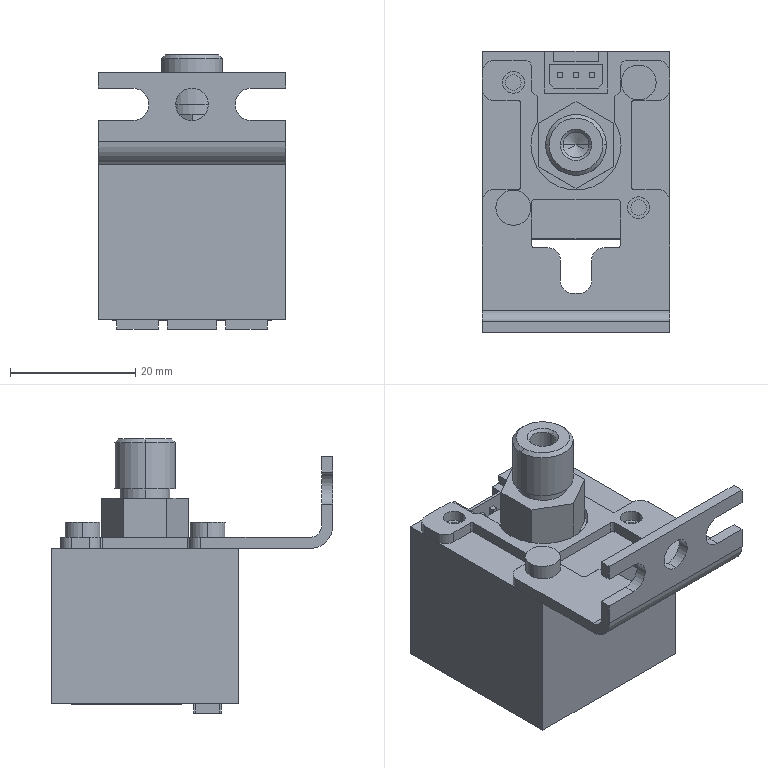Part | SolidWorks | features BaseBody 1 | 1 solid | 162 faces | box 30 x 45 x 43.8 mm | volume 25596 mm3 | plane 109 | cylinder 47 | cone 6 | commonest cylinder face diameters 4 x10 0.6 x4 1 x4 2.5 x4 3.5 x4 5.2 x4